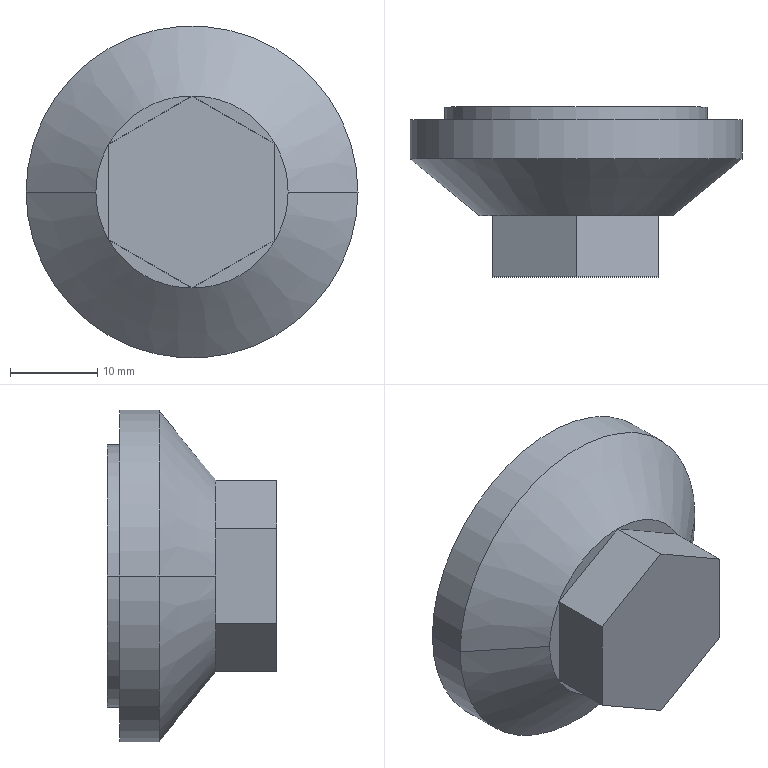Part | STEP file | LIB_58129429 | 1 solid | 28 faces | box 38 x 19.45 x 38 mm | volume 10239 mm3 | plane 14 | cylinder 12 | cone 2 | commonest cylinder face diameters 12 x2 20 x2 23.5 x2 30 x2 32 x2 38 x2